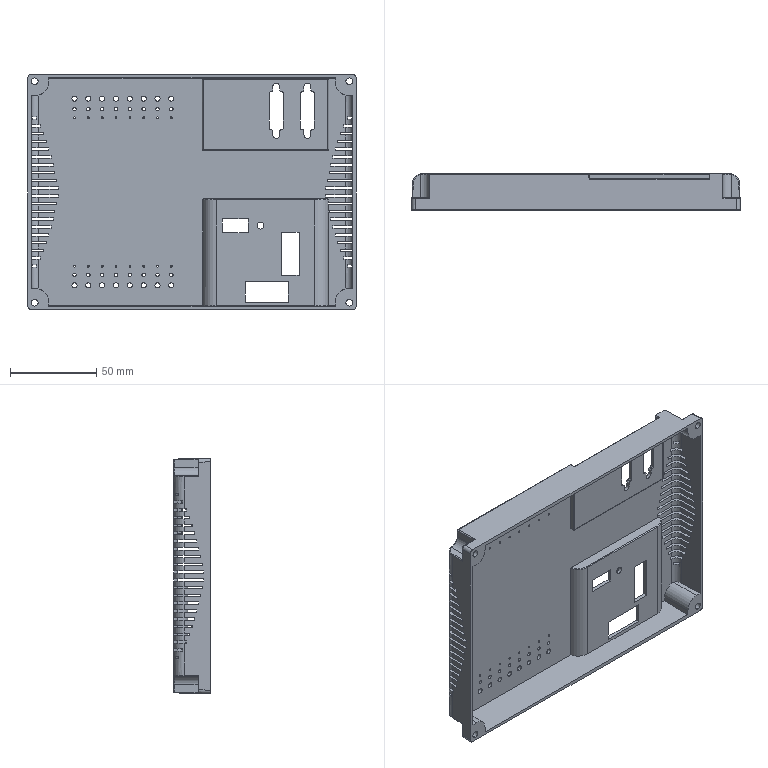Part | SolidWorks | features BaseBody 1 | 1 solid | 555 faces | box 190 x 21 x 136 mm | volume 72081 mm3 | cylinder 349 | plane 164 | spline 22 | torus 12 | sphere 8 | commonest cylinder face diameters 1 x77 12 x40 8 x38 2 x32 3 x32 4 x20